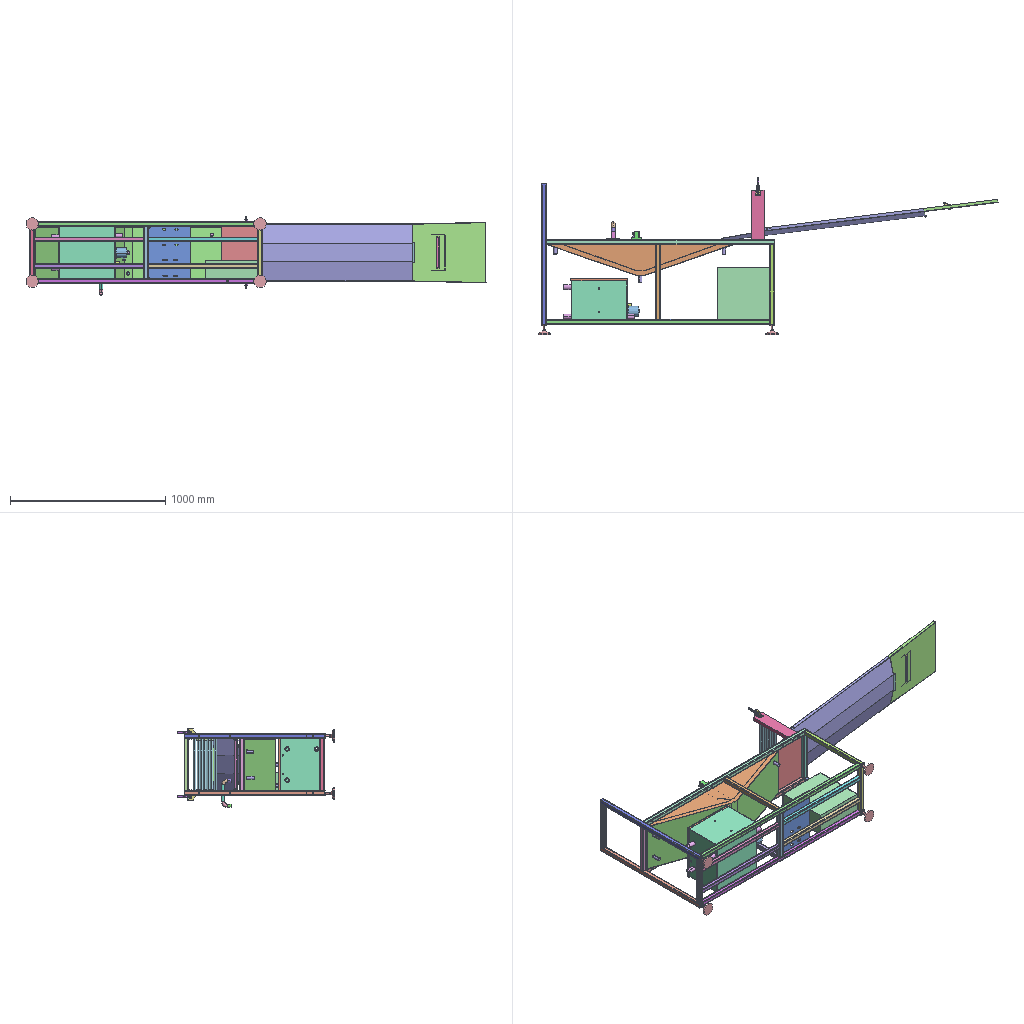Assembly | SolidWorks | 47 different items | 85 placed | box 2966 x 1014 x 507 mm
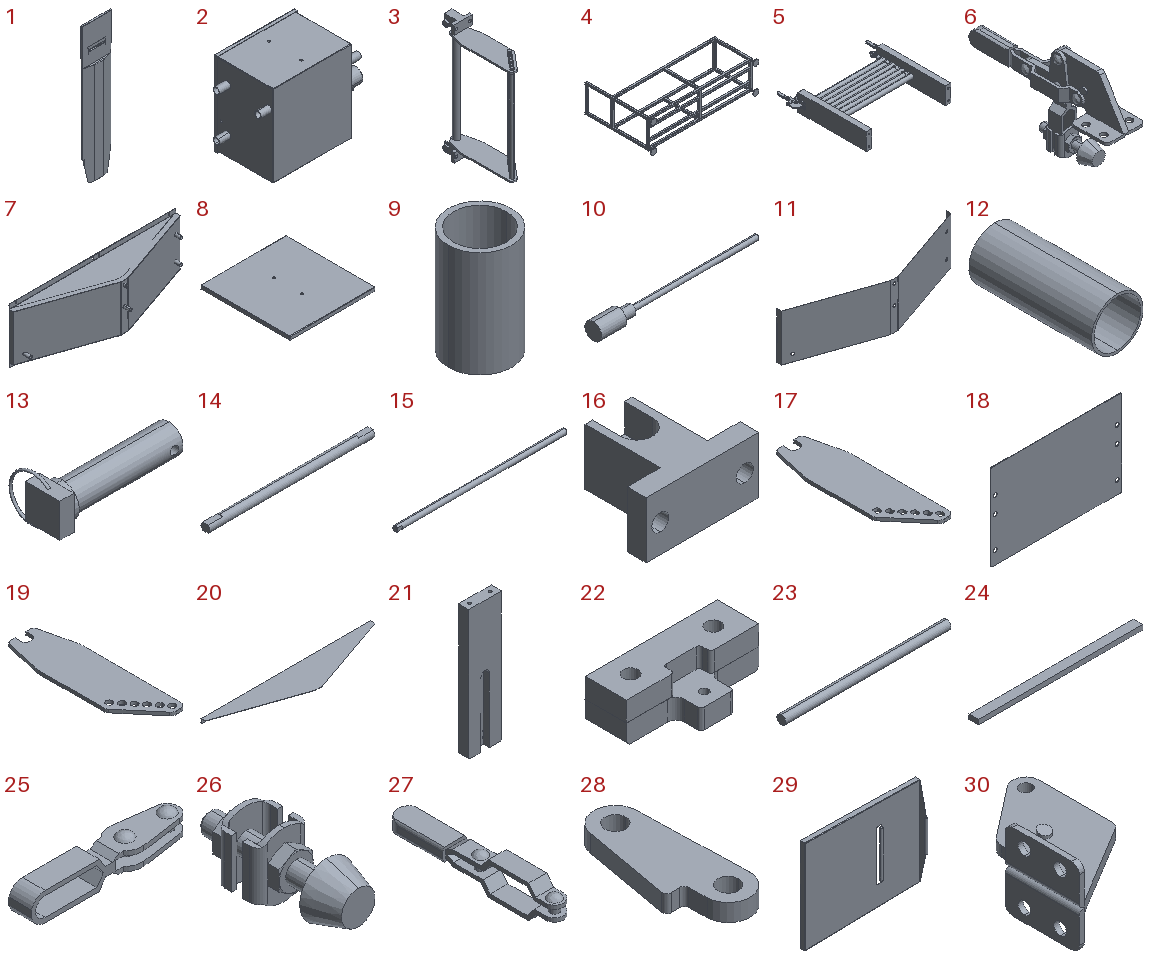Parts list (item | name | quantity | parent item | size | volume | features):
1 | (subassembly) | x1 | - | 389.95 x 79.837 x 1800 mm | 939174 mm3 | features AEMSimFeature 1, Fillet 1, RefAxis 1
2 | (subassembly) | x1 | - | 488 x 266.5 x 384 mm | 1398529 mm3 | features CompositeCurve 7
3 | (subassembly) | x1 | - | 68 x 246.296 x 400 mm | 467246 mm3 | features ReferencePattern 5, LocalLPattern 1
4 | (subassembly) | x1 | - | 1550 x 971 x 450 mm | 4239958 mm3 | features CompositeCurve 4, AEMSimFeature 1
5 | (subassembly) | x1 | - | 463.4 x 403.3 x 80 mm | 2031075 mm3 | features ReferencePattern 10, LocalLPattern 2, AEMSimFeature 1
6 | (subassembly) | x2 | in 5 | 30 x 119.8 x 70.25 mm | 20145 mm3 | features LocalCirPattern 1, ReferencePattern 1
7 | (subassembly) | x1 | - | 1200 x 275.844 x 398 mm | 2176223 mm3 | features CompositeCurve 3
8 | - | x1 | in 2 | 369 x 384 x 15 mm | 241174 mm3 | features EdgeFlange 1, FlatPattern 1, ICE 1, SMBaseFlange 1, SheetMetal 1
9 | - | x4 | in 2 | 30 x 30 x 50 mm | 10799 mm3 | features Extrusion 1
10 | - | x1 | in 2 | 195 x 20 x 20 mm | 15362 mm3 | features Revolution 1
11 | - | x1 | in 7 | 1200 x 230 x 330 mm | 522694 mm3 | features ICE 4, FlatPattern 1, SMBaseFlange 1, SheetMetal 1
12 | - | x5 | in 7 | 21 x 50 x 21 mm | 3142 mm3 | features Extrusion 1
13 | - | x2 | in 3 | 45 x 19.844 x 16.686 mm | 3901 mm3 | features ICE 3, BaseBody 1, Sweep 1
14 | - | x1 | in 3 | 374 x 20 x 20 mm | 115370 mm3 | features ICE 3, Extrusion 1, HoleWzd 1
15 | - | x6 | in 3 | 326 x 10 x 10 mm | 25495 mm3 | features HoleWzd 2, Chamfer 1, Extrusion 1, ICE 1
16 | - | x1 | in 3 | 60 x 50 x 30 mm | 40656 mm3 | features 3DProfileFeature 2, HoleWzd 2, Extrusion 1, ICE 1
17 | - | x1 | in 3 | 68 x 225 x 5 mm | 61691 mm3 | features Fillet 5, ICE 5, Extrusion 1, LPattern 1
18 | - | x1 | - | 398 x 1.5 x 262 mm | 155364 mm3 | features Fillet 1, FlatPattern 1, HoleWzd 1, SMBaseFlange 1, SheetMetal 1
19 | - | x1 | in 3 | 68 x 225 x 5 mm | 61427 mm3 | features Fillet 5, ICE 4, Extrusion 1
20 | - | x1 | in 7 | 1200 x 232 x 34 mm | 400369 mm3 | features MirrorStock 1
21 | - | x2 | in 5 | 80 x 25 x 320 mm | 584909 mm3 | features HoleWzd 3, ICE 3, Chamfer 1, Extrusion 1
22 | - | x1 | in 5 | 80 x 40 x 24 mm | 46437 mm3 | features ICE 5, Fillet 3, HoleWzd 2, Chamfer 1, Extrusion 1
23 | - | x7 | in 5 | 370 x 20 x 20 mm | 116239 mm3 | features ICE 1, MirrorPattern 1, Revolution 1
24 | - | x1 | in 5 | 345 x 20 x 10 mm | 69000 mm3 | features Extrusion 1
25 | - | x2 | in 6 | 70.05 x 15.001 x 12.4 mm | 3515 mm3 | features BaseBody 1
26 | - | x2 | in 6 | 16 x 44.45 x 19 mm | 3867 mm3 | features BaseBody 1
27 | - | x2 | in 6 | 12.6 x 89.5 x 17.6 mm | 5262 mm3 | features BaseBody 1
28 | - | x2 | in 6 | 14.127 x 35.318 x 4 mm | 1354 mm3 | features BaseBody 1
29 | - | x1 | in 1 | 480 x 56.239 x 389.95 mm | 276290 mm3 | features ICE 4, EdgeFlange 2, CornerFeat 1, Fillet 1, FlatPattern 1, SMBaseFlange 1, SheetMetal 1
30 | - | x2 | in 6 | 34.2 x 55.001 x 30 mm | 6148 mm3 | features BaseBody 1
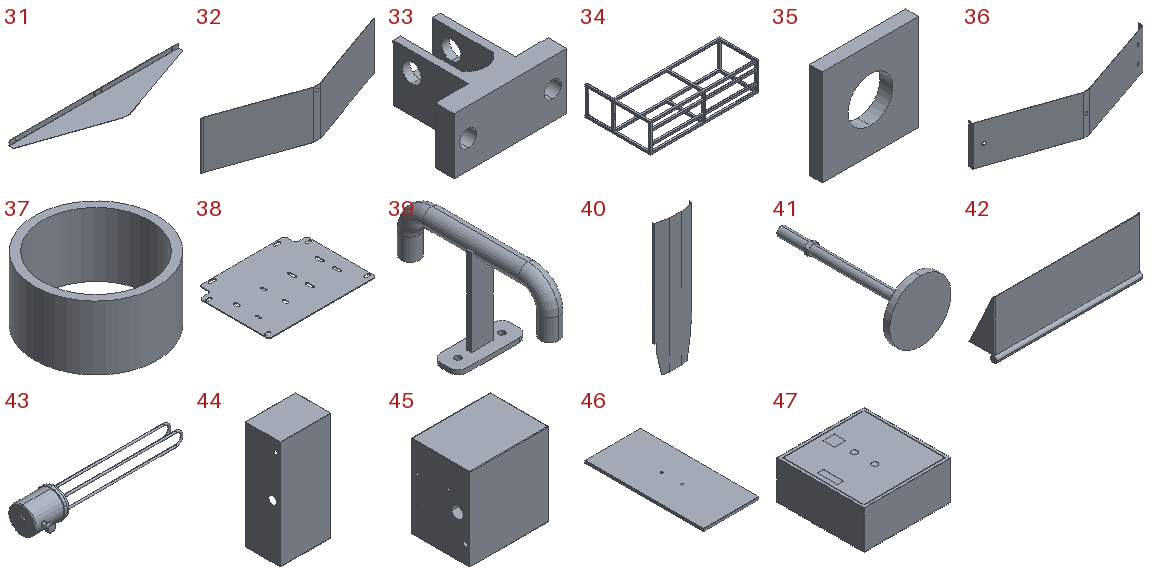31 | - | x1 | in 7 | 1200 x 232 x 34 mm | 400369 mm3 | features ICE 4, EdgeFlange 1, Fillet 1, FlatPattern 1, SMBaseFlange 1, SheetMetal 1
32 | - | x1 | in 7 | 1200 x 202 x 330 mm | 837082 mm3 | features ICE 2, Fillet 1, FlatPattern 1, SMBaseFlange 1, SheetMetal 1
33 | - | x2 | in 3 | 60 x 50 x 30 mm | 33992 mm3 | features BaseBody 1
34 | - | x1 | in 4 | 1500 x 905 x 400 mm | 3870748 mm3 | features WeldCornerFeat 8, HoleWzd 5, 3DProfileFeature 1, ICE 1, MirrorPattern 1, WeldMemberFeat 1, WeldmentFeature 1
35 | - | x4 | in 4 | 30 x 4 x 30 mm | 2984 mm3 | features ICE 2, Extrusion 1
36 | - | x1 | in 7 | 1200 x 230 x 280 mm | 738116 mm3 | features ICE 4, FlatPattern 1, SMBaseFlange 1, SheetMetal 1
37 | - | x6 | in 5 | 23 x 23 x 12 mm | 1216 mm3 | features Extrusion 1
38 | - | x1 | - | 400 x 300 x 3 mm | 340160 mm3 | features ICE 3, Extrusion 1, Fillet 1
39 | - | x1 | - | 80 x 181.3 x 115.65 mm | 40270 mm3 | features ICE 2, 3DProfileFeature 1, BossThin 1, Extrusion 1, Fillet 1, WeldMemberFeat 1, WeldmentFeature 1
40 | - | x1 | in 1 | 370 x 47.712 x 1320 mm | 619084 mm3 | features Fillet 3, ICE 2, FlatPattern 1, HoleWzd 1, SMBaseFlange 1, SheetMetal 1
41 | - | x4 | in 4 | 80 x 182 x 80 mm | 89449 mm3 | features ICE 6, Chamfer 1, Revolution 1
42 | - | x1 | in 1 | 230 x 44 x 90 mm | 43833 mm3 | features ICE 2, EdgeFlange 1, FlatPattern 1, SMBaseFlange 1, SheetMetal 1
43 | - | x1 | in 2 | 378 x 88 x 70 mm | 302343 mm3 | features ICE 6, Chamfer 1, CirPattern 1, Fillet 1, MirrorPattern 1, Revolution 1, Sweep 1
44 | - | x1 | in 2 | 362.4 x 253.2 x 776.2 mm | 1035495 mm3 | features ICE 8, EdgeFlange 4, 3DProfileFeature 3, HoleWzd 3, FlatPattern 1, SMBaseFlange 1, SheetMetal 1
45 | - | x1 | in 2 | 360 x 265 x 375 mm | 796453 mm3 | features ICE 7, EdgeFlange 2, FlatPattern 1, SMBaseFlange 1, SheetMetal 1
46 | - | x1 | in 2 | 328.4 x 698.4 x 15 mm | 307582 mm3 | features EdgeFlange 1, FlatPattern 1, ICE 1, SMBaseFlange 1, SheetMetal 1
47 | - | x1 | - | 340 x 340 x 151 mm | 586961 mm3 | features ICE 2, Extrusion 1, Shell 1
Mates (type | each side: item.copy, entity, surface, feature):
In the top assembly
Coincident | 34.1 face plane  D:\PROGRAM FILES\SOLIDWORKS CORP\SOLIDWORKS\LANG\CHINESE-SIMPLIFIED\WELDMENT PROFILES\SOLIDWORKS weldment profile library GB\square tube\30 X 30 X 2.6 - missing(2) | 31.1 face plane
Coincident | 34.1 face plane  D:\PROGRAM FILES\SOLIDWORKS CORP\SOLIDWORKS\LANG\CHINESE-SIMPLIFIED\WELDMENT PROFILES\SOLIDWORKS weldment profile library GB\square tube\30 X 30 X 2.6 - missing(2) | 21.1 face plane Boss-Extrude1
Concentric | 34.1 face cylinder M8 Clearance Hole1 | 21.2 face cylinder M8 Tapped Hole1 | 2 times
Width | 31.1 face plane | 20.1 face plane single outlet.SLY1235K.25.1 KYSESa glue groove side plate 1 SR_Mirror1 | 34.1 face plane | 34.1 face plane  D:\PROGRAM FILES\SOLIDWORKS CORP\SOLIDWORKS\LANG\CHINESE-SIMPLIFIED\WELDMENT PROFILES\SOLIDWORKS weldment profile library GB\square tube\30 X 30 X 2.6 - missing(2)
DistanceDim | 31.1 face plane | 34.1 face plane  D:\PROGRAM FILES\SOLIDWORKS CORP\SOLIDWORKS\LANG\CHINESE-SIMPLIFIED\WELDMENT PROFILES\SOLIDWORKS weldment profile library GB\square tube\30 X 30 X 2.6 - missing(2)
Coincident | 20.1 face plane single outlet.SLY1235K.25.1 KYSESa glue groove side plate 1 SR_Mirror1 | 33.1 face plane Import 1
Width | 20.1 face plane single outlet.SLY1235K.25.1 KYSESa glue groove side plate 1 SR_Mirror1 | 31.1 face plane | 17.1 face plane Boss-Extrude1 | 19.1 face plane Boss-Extrude1
Coincident | 34.1 face plane  D:\PROGRAM FILES\SOLIDWORKS CORP\SOLIDWORKS\LANG\CHINESE-SIMPLIFIED\WELDMENT PROFILES\SOLIDWORKS weldment profile library GB\square tube\30 X 30 X 2.6 - missing(2) | 45.1 face plane Base-Flange1
Width | 40.1 face plane | 40.1 face plane | 21.1 face plane Boss-Extrude1 | 21.2 face plane Boss-Extrude1
PlanarAngleDim | 29.1 face plane Base-Flange1 | 34.1 face plane  D:\PROGRAM FILES\SOLIDWORKS CORP\SOLIDWORKS\LANG\CHINESE-SIMPLIFIED\WELDMENT PROFILES\SOLIDWORKS weldment profile library GB\square tube\30 X 30 X 2.6 - missing(2)
Tangent | 32.1 face cylinder Base Bend 4 | 40.1 face plane
Coincident | 34.1 face plane | 18.1 face plane Base-Flange1
Width | 18.1 face plane Base-Flange1 | 18.1 face plane Base-Flange1 | 34.1 face plane  D:\PROGRAM FILES\SOLIDWORKS CORP\SOLIDWORKS\LANG\CHINESE-SIMPLIFIED\WELDMENT PROFILES\SOLIDWORKS weldment profile library GB\square tube\30 X 30 X 2.6 - missing(2) | 34.1 face plane
Concentric | 34.1 face cylinder | 18.1 edge
Coincident | 34.1 edge | 33.2 face cylinder Import 1
Width | 45.1 face plane Edge-Flange1 | 45.1 face plane Edge-Flange1 | 34.1 face plane  D:\PROGRAM FILES\SOLIDWORKS CORP\SOLIDWORKS\LANG\CHINESE-SIMPLIFIED\WELDMENT PROFILES\SOLIDWORKS weldment profile library GB\square tube\30 X 30 X 2.6 - missing(2) | 34.1 face plane  D:\PROGRAM FILES\SOLIDWORKS CORP\SOLIDWORKS\LANG\CHINESE-SIMPLIFIED\WELDMENT PROFILES\SOLIDWORKS weldment profile library GB\square tube\30 X 30 X 2.6 - missing(2)
Coincident | 34.1 face plane  D:\PROGRAM FILES\SOLIDWORKS CORP\SOLIDWORKS\LANG\CHINESE-SIMPLIFIED\WELDMENT PROFILES\SOLIDWORKS weldment profile library GB\square tube\30 X 30 X 2.6 - missing(2) | 38.1 face plane Boss-Extrude1 | 2 times
Width | 38.1 face plane Boss-Extrude1 | 38.1 face plane Boss-Extrude1 | 34.1 face plane  D:\PROGRAM FILES\SOLIDWORKS CORP\SOLIDWORKS\LANG\CHINESE-SIMPLIFIED\WELDMENT PROFILES\SOLIDWORKS weldment profile library GB\square tube\30 X 30 X 2.6 - missing(2) | 34.1 face plane  D:\PROGRAM FILES\SOLIDWORKS CORP\SOLIDWORKS\LANG\CHINESE-SIMPLIFIED\WELDMENT PROFILES\SOLIDWORKS weldment profile library GB\square tube\30 X 30 X 2.6 - missing(2)
Coincident | 34.1 face plane  D:\PROGRAM FILES\SOLIDWORKS CORP\SOLIDWORKS\LANG\CHINESE-SIMPLIFIED\WELDMENT PROFILES\SOLIDWORKS weldment profile library GB\square tube\30 X 30 X 2.6 - missing(2) | 47.1 face plane Boss-Extrude1 | 2 times
DistanceDim | 45.1 face plane Edge-Flange1 | 34.1 face plane  D:\PROGRAM FILES\SOLIDWORKS CORP\SOLIDWORKS\LANG\CHINESE-SIMPLIFIED\WELDMENT PROFILES\SOLIDWORKS weldment profile library GB\square tube\30 X 30 X 2.6 - missing(2)
Coincident | 31.1 face plane | 39.1 face plane Boss-Extrude1
Concentric | 31.1 face cylinder Cut-Extrude1 | 39.1 face cylinder Boss-Extrude1
Coincident | 34.1 face plane  D:\PROGRAM FILES\SOLIDWORKS CORP\SOLIDWORKS\LANG\CHINESE-SIMPLIFIED\WELDMENT PROFILES\SOLIDWORKS weldment profile library GB\square tube\30 X 30 X 2.6 - missing(2) | 47.1 face plane Boss-Extrude2
In subassembly 7
Concentric | 7.1 face | 32.2 face cylinder Cut-Extrude1
Coincident | 7.1 edge | 32.2 face plane Base-Flange1
Coincident | 7.1 face | 7.1 face | 3 times
Coincident | 31.2 face plane Edge-Flange1 | 7.1 face
Coincident | 32.2 face plane Base-Flange1 | 31.2 face plane Base-Flange1
Coincident | 32.2 face plane Base-Flange1 | 31.2 face plane Edge-Flange1 | 2 times
Coincident | 32.2 face plane Base-Flange1 | 20.2 face plane single outlet.SLY1235K.25.1 KYSESa glue groove side plate 1 SR_Mirror1
Coincident | 31.2 face plane Edge-Flange1 | 20.2 face plane single outlet.SLY1235K.25.1 KYSESa glue groove side plate 1 SR_Mirror1
Coincident | 31.2 face plane Base-Flange1 | 20.2 face plane single outlet.SLY1235K.25.1 KYSESa glue groove side plate 1 SR_Mirror1
Coincident | 32.2 face plane Base-Flange1 | 36.1 face plane Base-Flange1
Coincident | 20.2 face plane single outlet.SLY1235K.25.1 KYSESa glue groove side plate 1 SR_Mirror1 | 36.1 face plane Base-Flange1 | 2 times
Coincident | 36.1 face plane Base-Flange1 | 11.1 face plane Base-Flange1
Coincident | 31.2 face plane Edge-Flange1 | 11.1 face plane Base-Flange1
Tangent | 12.1 face cylinder Boss-Extrude1 | 11.1 edge
Concentric | 12.2 face cylinder Boss-Extrude1 | 11.1 edge
Concentric | 12.3 face cylinder Boss-Extrude1 | 11.1 face cylinder Cut-Extrude4
Concentric | 11.1 edge | 12.4 face cylinder Boss-Extrude1
Coincident | 32.2 face plane Base-Flange1 | 12.4 face plane Boss-Extrude1
Coincident | 31.2 face plane Base-Flange1 | 11.1 face plane Base-Flange1
In subassembly 3
Coincident | 3.1 face | 14.1 face plane Boss-Extrude1
Concentric | 3.1 face | 14.1 face cylinder Boss-Extrude1
Coincident | 14.1 face plane Boss-Extrude1 | 3.1 face
Coincident | 3.1 face | 3.1 face | 2 times
Concentric | 14.1 face cylinder Boss-Extrude1 | 3.1 face | 4 times
Concentric | 3.1 face | 3.1 face
PlanarAngleDim | 3.1 face | 3.1 face | 2 times
DistanceDim | 14.1 face plane Boss-Extrude1 | 3.1 face
Parallel | 14.1 face plane Cut-Extrude2 | 3.1 face
DistanceDim | 14.1 face plane Boss-Extrude1 | 16.1 face plane Cut-Extrude1
Coincident | 3.1 face | 16.1 face plane Boss-Extrude1 | 2 times
Concentric | 14.1 face cylinder Boss-Extrude1 | 19.2 face cylinder Cut-Extrude3
Concentric | 14.1 face cylinder Boss-Extrude1 | 17.2 face cylinder Cut-Extrude3
Concentric | 19.2 face cylinder Cut-Extrude1 | 17.2 face cylinder Cut-Extrude1
DistanceDim | 17.2 face plane Boss-Extrude1 | 19.2 face plane Boss-Extrude1
Width | 17.2 face plane Boss-Extrude1 | 19.2 face plane Boss-Extrude1 | 16.1 face plane Boss-Extrude1 | 3.1 face
Concentric | 15.1 face cylinder Boss-Extrude1 | 17.2 face cylinder Cut-Extrude1
Parallel | 15.1 face plane Cut-Extrude1 | 17.2 face plane LPattern1
Concentric | 14.1 face cylinder Boss-Extrude1 | 33.3 face cylinder Import 1
Parallel | 14.1 face plane Cut-Extrude1 | 33.3 face plane Import 1
Parallel | 3.1 face | 16.1 face plane Boss-Extrude1
Concentric | 14.1 face cylinder Boss-Extrude1 | 33.4 face cylinder Import 1
Parallel | 14.1 face plane Cut-Extrude2 | 33.4 face plane Import 1
Width | 33.4 face plane Import 1 | 33.3 face plane Import 1 | 19.2 face plane Boss-Extrude1 | 17.2 face plane Boss-Extrude1
DistanceDim | 33.4 face plane Import 1 | 33.3 face plane Import 1
Concentric | 33.4 face cylinder Import 1 | 13.1 face cylinder Import 1
Coincident | 33.4 face plane Import 1 | 13.1 face plane Import 1
Coincident | 33.3 face plane Import 1 | 13.2 face plane Import 1
Concentric | 33.3 face cylinder Import 1 | 13.2 face cylinder Import 1
Width | 14.1 face plane Boss-Extrude1 | 14.1 face plane Boss-Extrude1 | 33.4 face plane Import 1 | 33.3 face plane Import 1
DistanceDim | 15.1 face plane Boss-Extrude1 | 17.2 face plane Boss-Extrude1
Parallel | 14.1 face plane Cut-Extrude1 | 17.2 face plane Cut-Extrude3
Coincident | 16.1 face plane Boss-Extrude1 | 33.4 face plane Import 1 | 2 times
In subassembly 4
Coincident | 35.1 face plane Boss-Extrude1 | 35.2 face plane Boss-Extrude1 | 2 times
Coincident | 35.1 face plane Boss-Extrude1 | 35.3 face plane Boss-Extrude1 | 2 times
Coincident | 35.3 face plane Boss-Extrude1 | 35.4 face plane Boss-Extrude1 | 2 times
Coincident | 35.1 face plane Boss-Extrude1 | 34.2 face plane  D:\PROGRAM FILES\SOLIDWORKS CORP\SOLIDWORKS\LANG\CHINESE-SIMPLIFIED\WELDMENT PROFILES\SOLIDWORKS weldment profile library GB\square tube\30 X 30 X 2.6 - missing(2)
Coincident | 34.2 face plane  D:\PROGRAM FILES\SOLIDWORKS CORP\SOLIDWORKS\LANG\CHINESE-SIMPLIFIED\WELDMENT PROFILES\SOLIDWORKS weldment profile library GB\square tube\30 X 30 X 2.6 - missing(2) | 35.1 face plane Boss-Extrude1 | 2 times
Coincident | 34.2 face plane  D:\PROGRAM FILES\SOLIDWORKS CORP\SOLIDWORKS\LANG\CHINESE-SIMPLIFIED\WELDMENT PROFILES\SOLIDWORKS weldment profile library GB\square tube\30 X 30 X 2.6 - missing(2) | 35.3 face plane Boss-Extrude1
Coincident | 34.2 face plane  D:\PROGRAM FILES\SOLIDWORKS CORP\SOLIDWORKS\LANG\CHINESE-SIMPLIFIED\WELDMENT PROFILES\SOLIDWORKS weldment profile library GB\square tube\30 X 30 X 2.6 - missing(2) | 35.2 face plane Boss-Extrude1
Coincident | 35.4 face plane Boss-Extrude1 | 35.2 face plane Boss-Extrude1
Concentric | 35.1 edge | 41.1 face cylinder Revolve1
DistanceDim | 35.1 face plane Boss-Extrude1 | 41.1 face plane Boss-Extrude1
Concentric | 35.2 edge | 41.2 face cylinder Revolve1
Coincident | 41.1 face plane Revolve1 | 41.2 face plane Revolve1
Concentric | 35.3 edge | 41.3 face cylinder Revolve1
Concentric | 35.4 edge | 41.4 face cylinder Revolve1
Coincident | 41.2 face plane Revolve1 | 41.4 face plane Revolve1
Coincident | 41.1 face plane Revolve1 | 41.3 face plane Revolve1
In subassembly 5
DistanceDim | 21.3 face plane Boss-Extrude1 | 21.4 face plane Boss-Extrude1
Width | 21.3 face plane Boss-Extrude1 | 21.4 face plane Boss-Extrude1 | 23.1 face plane Mirror1 | 23.1 face plane Revolve1
Coincident | 21.4 face plane Boss-Extrude1 | 30.1 face plane Import 1
Width | 30.1 face plane Import 1 | 30.1 face plane Import 1 | 21.4 face plane Boss-Extrude1 | 21.4 face plane Boss-Extrude1
DistanceDim | 30.1 face plane Import 1 | 21.4 face plane Boss-Extrude1
Coincident | 21.3 face plane Boss-Extrude1 | 30.2 face plane Import 1
Coincident | 30.1 face plane Import 1 | 30.2 face plane Import 1 | 2 times
Coincident | 21.4 face plane Boss-Extrude1 | 5.1 face | 2 times
DistanceDim | 21.4 face plane Boss-Extrude1 | 5.1 face
Concentric | 23.1 face cylinder Revolve1 | 21.4 face cylinder Cut-Extrude2
Coincident | 21.4 face plane Boss-Extrude1 | 21.3 face plane Boss-Extrude1 | 2 times
Coincident | 21.4 face plane Boss-Extrude1 | 22.1 face | 3 times
Coincident | 21.3 face plane Boss-Extrude1 | 22.2 face | 3 times
Concentric | 23.2 face cylinder Revolve1 | 37.1 face cylinder Boss-Extrude1
Concentric | 23.2 face cylinder Revolve1 | 37.2 face cylinder Boss-Extrude1
DistanceDim | 37.1 face plane Boss-Extrude1 | 21.4 face plane Boss-Extrude1
DistanceDim | 37.2 face plane Boss-Extrude1 | 21.3 face plane Boss-Extrude1
Coincident | 21.4 face plane Boss-Extrude1 | 24.1 face | 2 times
Coincident | 21.3 face plane Boss-Extrude1 | 24.2 face | 2 times
DistanceDim | 21.3 face plane Boss-Extrude1 | 24.2 face
Coincident | 21.3 face plane Boss-Extrude1 | 24.1 face
In subassembly 2
DistanceDim | 44.1 face | 2.1 face | 3 times
Coincident | 2.1 face | 2.1 face | 2 times
DistanceDim | 2.1 face | 2.1 face | 4 times
Coincident | 44.1 face | 46.1 face | 3 times
Concentric | 44.1 face | 43.1 face cylinder Boss-Extrude1
Coincident | 44.1 face | 43.1 face plane Revolve1
Concentric | 44.1 face | 2.1 face
Coincident | 44.1 face | 2.1 face
Coincident | 44.1 face | 9.1 face plane Boss-Extrude1
Concentric | 44.1 face | 9.1 face cylinder Boss-Extrude1
Coincident | 44.1 face | 9.2 face
Concentric | 44.1 face | 9.2 face
Coincident | 44.1 face | 9.3 face plane Boss-Extrude1
Coincident | 44.1 face | 9.4 face plane Boss-Extrude1
Concentric | 44.1 face | 9.4 face cylinder Boss-Extrude1
Coincident | 44.1 face | 10.1 face plane Revolve1
Concentric | 44.1 face | 10.1 face cylinder Revolve1
Concentric | 44.1 face | 9.3 face cylinder Boss-Extrude1
Coincident | 44.1 face | 9.5 face plane Boss-Extrude1
Concentric | 44.1 face | 9.5 face cylinder Boss-Extrude1
Coincident | 44.1 face | 45.2 face plane Base-Flange1
Coincident | 44.1 face | 45.2 face plane Edge-Flange1 | 2 times
Coincident | 45.2 face plane Edge-Flange2 | 8.1 face plane Base-Flange1
Width | 8.1 face plane Edge-Flange1 | 8.1 face plane Edge-Flange1 | 45.2 face plane Edge-Flange1 | 45.2 face plane Edge-Flange1
Width | 45.2 face plane Edge-Flange1 | 45.2 face plane Edge-Flange1 | 8.1 face plane Edge-Flange1 | 8.1 face plane Edge-Flange1
Concentric | 43.1 face cylinder Revolve1 | 45.2 edge
Concentric | 10.1 face cylinder Revolve1 | 45.2 edge
Coincident | 10.1 face plane Revolve1 | 45.2 face plane Edge-Flange1
Coincident | 43.1 face plane Revolve1 | 45.2 face plane Edge-Flange1
Concentric | 9.4 face cylinder Boss-Extrude1 | 45.2 edge
Coincident | 9.4 face plane Boss-Extrude1 | 45.2 face plane Edge-Flange1
Concentric | 9.1 face cylinder Boss-Extrude1 | 45.2 edge
Coincident | 9.1 face plane Boss-Extrude1 | 45.2 face plane Edge-Flange1
Concentric | 9.3 face cylinder Boss-Extrude1 | 45.2 edge
Coincident | 9.3 face plane Boss-Extrude1 | 45.2 face plane Edge-Flange1
Concentric | 9.5 face cylinder Boss-Extrude1 | 45.2 edge
Coincident | 9.5 face plane Boss-Extrude1 | 45.2 face plane Edge-Flange1
In subassembly 1
Coincident | 40.2 face plane | 29.2 face plane Edge-Flange2
Width | 29.2 face plane Edge-Flange1 | 29.2 face plane Edge-Flange1 | 40.2 face plane | 40.2 face plane
Coincident | 29.2 face plane Base-Flange1 | 42.1 face plane Cut-Extrude1
Width | 40.2 face plane | 40.2 face plane | 42.1 face plane Edge-Flange1 | 42.1 face plane Edge-Flange1
DistanceDim | 42.1 edge | 29.2 edge
Coincident | 40.2 face plane | 29.2 face plane Edge-Flange1